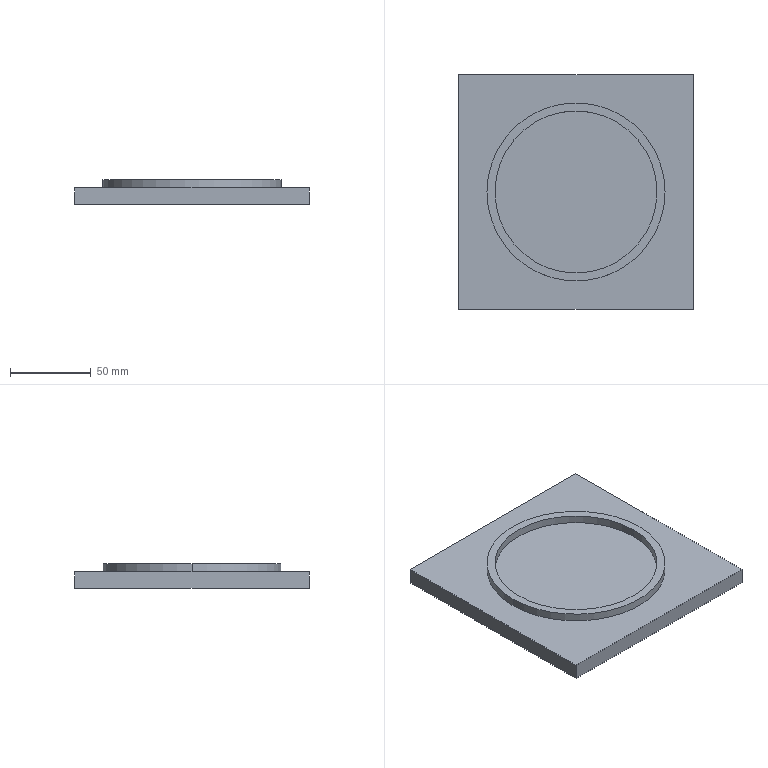Part | SolidWorks | features Extrusion 1, ICE 1 | 1 solid | 12 faces | box 145 x 145 x 15 mm | volume 218497 mm3 | plane 8 | cylinder 4 | commonest cylinder face diameters 100 x2 110 x2
STEP:
#1=CARTESIAN_POINT('',(22.5,72.5,15.));
#2=VERTEX_POINT('',#1);
#3=CARTESIAN_POINT('',(122.5,72.5,15.));
#4=VERTEX_POINT('',#3);
#5=CARTESIAN_POINT('',(72.5,72.5,15.));
#6=DIRECTION('',(0.,0.,1.));
#7=DIRECTION('',(1.,0.,0.));
#8=AXIS2_PLACEMENT_3D('',#5,#6,#7);
#9=CIRCLE('',#8,50.);
#10=EDGE_CURVE('',#2,#4,#9,.T.);
#11=ORIENTED_EDGE('',*,*,#10,.T.);
#12=CARTESIAN_POINT('',(122.5,72.5,10.));
#13=VERTEX_POINT('',#12);
#14=CARTESIAN_POINT('',(122.5,72.5,15.));
#15=DIRECTION('',(0.,0.,-1.));
#16=VECTOR('',#15,1000.);
#17=LINE('',#14,#16);
#18=EDGE_CURVE('',#4,#13,#17,.T.);
#19=ORIENTED_EDGE('',*,*,#18,.T.);
#20=CARTESIAN_POINT('',(22.5,72.5,10.));
#21=VERTEX_POINT('',#20);
#22=CARTESIAN_POINT('',(72.5,72.5,10.));
#23=DIRECTION('',(0.,0.,1.));
#24=DIRECTION('',(1.,0.,0.));
#25=AXIS2_PLACEMENT_3D('',#22,#23,#24);
#26=CIRCLE('',#25,50.);
#27=EDGE_CURVE('',#21,#13,#26,.T.);
#28=ORIENTED_EDGE('',*,*,#27,.F.);
#29=CARTESIAN_POINT('',(22.5,72.5,15.));
#30=DIRECTION('',(0.,0.,-1.));
#31=VECTOR('',#30,1000.);
#32=LINE('',#29,#31);
#33=EDGE_CURVE('',#2,#21,#32,.T.);
#34=ORIENTED_EDGE('',*,*,#33,.F.);
#35=EDGE_LOOP('',(#11,#19,#28,#34));
#36=FACE_OUTER_BOUND('',#35,.T.);
#37=CARTESIAN_POINT('',(72.5,72.5,15.));
#38=DIRECTION('',(0.,0.,-1.));
#39=DIRECTION('',(-1.,0.,0.));
#40=AXIS2_PLACEMENT_3D('',#37,#38,#39);
#41=CYLINDRICAL_SURFACE('',#40,50.);
#42=ADVANCED_FACE('',(#36),#41,.F.);
#43=CARTESIAN_POINT('',(127.5,72.5,15.));
#44=VERTEX_POINT('',#43);
#45=CARTESIAN_POINT('',(17.5,72.5,15.));
#46=VERTEX_POINT('',#45);
#47=CARTESIAN_POINT('',(72.5,72.5,15.));
#48=DIRECTION('',(0.,0.,1.));
#49=DIRECTION('',(1.,0.,0.));
#50=AXIS2_PLACEMENT_3D('',#47,#48,#49);
#51=CIRCLE('',#50,55.);
#52=EDGE_CURVE('',#44,#46,#51,.T.);
#53=ORIENTED_EDGE('',*,*,#52,.F.);
#54=CARTESIAN_POINT('',(127.5,72.5,10.));
#55=VERTEX_POINT('',#54);
#56=CARTESIAN_POINT('',(127.5,72.5,15.));
#57=DIRECTION('',(0.,0.,-1.));
#58=VECTOR('',#57,1000.);
#59=LINE('',#56,#58);
#60=EDGE_CURVE('',#44,#55,#59,.T.);
#61=ORIENTED_EDGE('',*,*,#60,.T.);
#62=CARTESIAN_POINT('',(17.5,72.5,10.));
#63=VERTEX_POINT('',#62);
#64=CARTESIAN_POINT('',(72.5,72.5,10.));
#65=DIRECTION('',(0.,0.,1.));
#66=DIRECTION('',(-1.,0.,0.));
#67=AXIS2_PLACEMENT_3D('',#64,#65,#66);
#68=CIRCLE('',#67,55.);
#69=EDGE_CURVE('',#55,#63,#68,.T.);
#70=ORIENTED_EDGE('',*,*,#69,.T.);
#71=CARTESIAN_POINT('',(17.5,72.5,15.));
#72=DIRECTION('',(0.,0.,-1.));
#73=VECTOR('',#72,1000.);
#74=LINE('',#71,#73);
#75=EDGE_CURVE('',#46,#63,#74,.T.);
#76=ORIENTED_EDGE('',*,*,#75,.F.);
#77=EDGE_LOOP('',(#53,#61,#70,#76));
#78=FACE_OUTER_BOUND('',#77,.T.);
#79=CARTESIAN_POINT('',(72.5,72.5,15.));
#80=DIRECTION('',(0.,0.,-1.));
#81=DIRECTION('',(-1.,0.,0.));
#82=AXIS2_PLACEMENT_3D('',#79,#80,#81);
#83=CYLINDRICAL_SURFACE('',#82,55.);
#84=ADVANCED_FACE('',(#78),#83,.T.);
#85=CARTESIAN_POINT('',(0.,145.,10.));
#86=VERTEX_POINT('',#85);
#87=CARTESIAN_POINT('',(0.,0.,10.));
#88=VERTEX_POINT('',#87);
#89=CARTESIAN_POINT('',(0.,0.,10.));
#90=DIRECTION('',(0.,-1.,0.));
#91=VECTOR('',#90,1000.);
#92=LINE('',#89,#91);
#93=EDGE_CURVE('',#86,#88,#92,.T.);
#94=ORIENTED_EDGE('',*,*,#93,.T.);
#95=CARTESIAN_POINT('',(145.,0.,10.));
#96=VERTEX_POINT('',#95);
#97=CARTESIAN_POINT('',(0.,0.,10.));
#98=DIRECTION('',(1.,0.,0.));
#99=VECTOR('',#98,1000.);
#100=LINE('',#97,#99);
#101=EDGE_CURVE('',#88,#96,#100,.T.);
#102=ORIENTED_EDGE('',*,*,#101,.T.);
#103=CARTESIAN_POINT('',(145.,145.,10.));
#104=VERTEX_POINT('',#103);
#105=CARTESIAN_POINT('',(145.,145.,10.));
#106=DIRECTION('',(0.,1.,0.));
#107=VECTOR('',#106,1000.);
#108=LINE('',#105,#107);
#109=EDGE_CURVE('',#96,#104,#108,.T.);
#110=ORIENTED_EDGE('',*,*,#109,.T.);
#111=CARTESIAN_POINT('',(0.,145.,10.));
#112=DIRECTION('',(-1.,0.,0.));
#113=VECTOR('',#112,1000.);
#114=LINE('',#111,#113);
#115=EDGE_CURVE('',#104,#86,#114,.T.);
#116=ORIENTED_EDGE('',*,*,#115,.T.);
#117=EDGE_LOOP('',(#94,#102,#110,#116));
#118=FACE_OUTER_BOUND('',#117,.T.);
#119=CARTESIAN_POINT('',(72.5,72.5,10.));
#120=DIRECTION('',(0.,0.,1.));
#121=DIRECTION('',(-1.,0.,0.));
#122=AXIS2_PLACEMENT_3D('',#119,#120,#121);
#123=CIRCLE('',#122,55.);
#124=EDGE_CURVE('',#63,#55,#123,.T.);
#125=ORIENTED_EDGE('',*,*,#124,.F.);
#126=ORIENTED_EDGE('',*,*,#69,.F.);
#127=EDGE_LOOP('',(#125,#126));
#128=FACE_BOUND('',#127,.T.);
#129=CARTESIAN_POINT('',(0.,145.,10.));
#130=DIRECTION('',(0.,0.,-1.));
#131=DIRECTION('',(-1.,0.,0.));
#132=AXIS2_PLACEMENT_3D('',#129,#130,#131);
#133=PLANE('',#132);
#134=ADVANCED_FACE('',(#118,#128),#133,.F.);
#135=CARTESIAN_POINT('',(0.,145.,0.));
#136=VERTEX_POINT('',#135);
#137=CARTESIAN_POINT('',(0.,0.,0.));
#138=VERTEX_POINT('',#137);
#139=CARTESIAN_POINT('',(0.,0.,0.));
#140=DIRECTION('',(0.,-1.,0.));
#141=VECTOR('',#140,1000.);
#142=LINE('',#139,#141);
#143=EDGE_CURVE('',#136,#138,#142,.T.);
#144=ORIENTED_EDGE('',*,*,#143,.T.);
#145=CARTESIAN_POINT('',(0.,0.,10.));
#146=DIRECTION('',(0.,0.,-1.));
#147=VECTOR('',#146,1000.);
#148=LINE('',#145,#147);
#149=EDGE_CURVE('',#88,#138,#148,.T.);
#150=ORIENTED_EDGE('',*,*,#149,.F.);
#151=ORIENTED_EDGE('',*,*,#93,.F.);
#152=CARTESIAN_POINT('',(0.,145.,10.));
#153=DIRECTION('',(0.,0.,-1.));
#154=VECTOR('',#153,1000.);
#155=LINE('',#152,#154);
#156=EDGE_CURVE('',#86,#136,#155,.T.);
#157=ORIENTED_EDGE('',*,*,#156,.T.);
#158=EDGE_LOOP('',(#144,#150,#151,#157));
#159=FACE_OUTER_BOUND('',#158,.T.);
#160=CARTESIAN_POINT('',(0.,0.,10.));
#161=DIRECTION('',(1.,0.,0.));
#162=DIRECTION('',(0.,0.,-1.));
#163=AXIS2_PLACEMENT_3D('',#160,#161,#162);
#164=PLANE('',#163);
#165=ADVANCED_FACE('',(#159),#164,.F.);
#166=CARTESIAN_POINT('',(145.,0.,0.));
#167=VERTEX_POINT('',#166);
#168=CARTESIAN_POINT('',(0.,0.,0.));
#169=DIRECTION('',(1.,0.,0.));
#170=VECTOR('',#169,1000.);
#171=LINE('',#168,#170);
#172=EDGE_CURVE('',#138,#167,#171,.T.);
#173=ORIENTED_EDGE('',*,*,#172,.T.);
#174=CARTESIAN_POINT('',(145.,0.,10.));
#175=DIRECTION('',(0.,0.,-1.));
#176=VECTOR('',#175,1000.);
#177=LINE('',#174,#176);
#178=EDGE_CURVE('',#96,#167,#177,.T.);
#179=ORIENTED_EDGE('',*,*,#178,.F.);
#180=ORIENTED_EDGE('',*,*,#101,.F.);
#181=ORIENTED_EDGE('',*,*,#149,.T.);
#182=EDGE_LOOP('',(#173,#179,#180,#181));
#183=FACE_OUTER_BOUND('',#182,.T.);
#184=CARTESIAN_POINT('',(0.,0.,10.));
#185=DIRECTION('',(0.,1.,0.));
#186=DIRECTION('',(0.,0.,1.));
#187=AXIS2_PLACEMENT_3D('',#184,#185,#186);
#188=PLANE('',#187);
#189=ADVANCED_FACE('',(#183),#188,.F.);
#190=CARTESIAN_POINT('',(145.,145.,0.));
#191=VERTEX_POINT('',#190);
#192=CARTESIAN_POINT('',(145.,145.,0.));
#193=DIRECTION('',(0.,1.,0.));
#194=VECTOR('',#193,1000.);
#195=LINE('',#192,#194);
#196=EDGE_CURVE('',#167,#191,#195,.T.);
#197=ORIENTED_EDGE('',*,*,#196,.T.);
#198=CARTESIAN_POINT('',(145.,145.,10.));
#199=DIRECTION('',(0.,0.,-1.));
#200=VECTOR('',#199,1000.);
#201=LINE('',#198,#200);
#202=EDGE_CURVE('',#104,#191,#201,.T.);
#203=ORIENTED_EDGE('',*,*,#202,.F.);
#204=ORIENTED_EDGE('',*,*,#109,.F.);
#205=ORIENTED_EDGE('',*,*,#178,.T.);
#206=EDGE_LOOP('',(#197,#203,#204,#205));
#207=FACE_OUTER_BOUND('',#206,.T.);
#208=CARTESIAN_POINT('',(145.,145.,10.));
#209=DIRECTION('',(-1.,0.,0.));
#210=DIRECTION('',(0.,-1.,0.));
#211=AXIS2_PLACEMENT_3D('',#208,#209,#210);
#212=PLANE('',#211);
#213=ADVANCED_FACE('',(#207),#212,.F.);
#214=CARTESIAN_POINT('',(0.,145.,0.));
#215=DIRECTION('',(-1.,0.,0.));
#216=VECTOR('',#215,1000.);
#217=LINE('',#214,#216);
#218=EDGE_CURVE('',#191,#136,#217,.T.);
#219=ORIENTED_EDGE('',*,*,#218,.T.);
#220=ORIENTED_EDGE('',*,*,#156,.F.);
#221=ORIENTED_EDGE('',*,*,#115,.F.);
#222=ORIENTED_EDGE('',*,*,#202,.T.);
#223=EDGE_LOOP('',(#219,#220,#221,#222));
#224=FACE_OUTER_BOUND('',#223,.T.);
#225=CARTESIAN_POINT('',(0.,145.,10.));
#226=DIRECTION('',(0.,-1.,0.));
#227=DIRECTION('',(0.,0.,-1.));
#228=AXIS2_PLACEMENT_3D('',#225,#226,#227);
#229=PLANE('',#228);
#230=ADVANCED_FACE('',(#224),#229,.F.);
#231=ORIENTED_EDGE('',*,*,#143,.F.);
#232=ORIENTED_EDGE('',*,*,#218,.F.);
#233=ORIENTED_EDGE('',*,*,#196,.F.);
#234=ORIENTED_EDGE('',*,*,#172,.F.);
#235=EDGE_LOOP('',(#231,#232,#233,#234));
#236=FACE_OUTER_BOUND('',#235,.T.);
#237=CARTESIAN_POINT('',(0.,145.,0.));
#238=DIRECTION('',(0.,0.,-1.));
#239=DIRECTION('',(-1.,0.,0.));
#240=AXIS2_PLACEMENT_3D('',#237,#238,#239);
#241=PLANE('',#240);
#242=ADVANCED_FACE('',(#236),#241,.T.);
#243=CARTESIAN_POINT('',(72.5,72.5,15.));
#244=DIRECTION('',(0.,0.,1.));
#245=DIRECTION('',(1.,0.,0.));
#246=AXIS2_PLACEMENT_3D('',#243,#244,#245);
#247=CIRCLE('',#246,55.);
#248=EDGE_CURVE('',#46,#44,#247,.T.);
#249=ORIENTED_EDGE('',*,*,#248,.T.);
#250=ORIENTED_EDGE('',*,*,#52,.T.);
#251=EDGE_LOOP('',(#249,#250));
#252=FACE_OUTER_BOUND('',#251,.T.);
#253=ORIENTED_EDGE('',*,*,#10,.F.);
#254=CARTESIAN_POINT('',(72.5,72.5,15.));
#255=DIRECTION('',(0.,0.,1.));
#256=DIRECTION('',(1.,0.,0.));
#257=AXIS2_PLACEMENT_3D('',#254,#255,#256);
#258=CIRCLE('',#257,50.);
#259=EDGE_CURVE('',#4,#2,#258,.T.);
#260=ORIENTED_EDGE('',*,*,#259,.F.);
#261=EDGE_LOOP('',(#253,#260));
#262=FACE_BOUND('',#261,.T.);
#263=CARTESIAN_POINT('',(72.5,72.5,15.));
#264=DIRECTION('',(0.,0.,1.));
#265=DIRECTION('',(1.,0.,0.));
#266=AXIS2_PLACEMENT_3D('',#263,#264,#265);
#267=PLANE('',#266);
#268=ADVANCED_FACE('',(#252,#262),#267,.T.);
#269=ORIENTED_EDGE('',*,*,#60,.F.);
#270=ORIENTED_EDGE('',*,*,#248,.F.);
#271=ORIENTED_EDGE('',*,*,#75,.T.);
#272=ORIENTED_EDGE('',*,*,#124,.T.);
#273=EDGE_LOOP('',(#269,#270,#271,#272));
#274=FACE_OUTER_BOUND('',#273,.T.);
#275=CARTESIAN_POINT('',(72.5,72.5,15.));
#276=DIRECTION('',(0.,0.,-1.));
#277=DIRECTION('',(-1.,0.,0.));
#278=AXIS2_PLACEMENT_3D('',#275,#276,#277);
#279=CYLINDRICAL_SURFACE('',#278,55.);
#280=ADVANCED_FACE('',(#274),#279,.T.);
#281=ORIENTED_EDGE('',*,*,#18,.F.);
#282=ORIENTED_EDGE('',*,*,#259,.T.);
#283=ORIENTED_EDGE('',*,*,#33,.T.);
#284=CARTESIAN_POINT('',(72.5,72.5,10.));
#285=DIRECTION('',(0.,0.,1.));
#286=DIRECTION('',(1.,0.,0.));
#287=AXIS2_PLACEMENT_3D('',#284,#285,#286);
#288=CIRCLE('',#287,50.);
#289=EDGE_CURVE('',#13,#21,#288,.T.);
#290=ORIENTED_EDGE('',*,*,#289,.F.);
#291=EDGE_LOOP('',(#281,#282,#283,#290));
#292=FACE_OUTER_BOUND('',#291,.T.);
#293=CARTESIAN_POINT('',(72.5,72.5,15.));
#294=DIRECTION('',(0.,0.,-1.));
#295=DIRECTION('',(-1.,0.,0.));
#296=AXIS2_PLACEMENT_3D('',#293,#294,#295);
#297=CYLINDRICAL_SURFACE('',#296,50.);
#298=ADVANCED_FACE('',(#292),#297,.F.);
#299=ORIENTED_EDGE('',*,*,#27,.T.);
#300=ORIENTED_EDGE('',*,*,#289,.T.);
#301=EDGE_LOOP('',(#299,#300));
#302=FACE_OUTER_BOUND('',#301,.T.);
#303=CARTESIAN_POINT('',(0.,145.,10.));
#304=DIRECTION('',(0.,0.,-1.));
#305=DIRECTION('',(-1.,0.,0.));
#306=AXIS2_PLACEMENT_3D('',#303,#304,#305);
#307=PLANE('',#306);
#308=ADVANCED_FACE('',(#302),#307,.F.);
#309=CLOSED_SHELL('',(#42,#84,#134,#165,#189,#213,#230,#242,#268,#280,#298,#308));
#310=MANIFOLD_SOLID_BREP('',#309);
#311=CARTESIAN_POINT('',(0.,0.,0.));
#312=DIRECTION('',(0.,0.,1.));
#313=DIRECTION('',(1.,0.,0.));
#314=AXIS2_PLACEMENT_3D('',#311,#312,#313);
#315=(LENGTH_UNIT()NAMED_UNIT(*)SI_UNIT(.MILLI.,.METRE.));
#316=UNCERTAINTY_MEASURE_WITH_UNIT(LENGTH_MEASURE(0.00001),#315,'','');
#317=(NAMED_UNIT(*)PLANE_ANGLE_UNIT()SI_UNIT($,.RADIAN.));
#318=(NAMED_UNIT(*)SI_UNIT($,.STERADIAN.)SOLID_ANGLE_UNIT());
#319=(GEOMETRIC_REPRESENTATION_CONTEXT(3)GLOBAL_UNCERTAINTY_ASSIGNED_CONTEXT((#316))GLOBAL_UNIT_ASSIGNED_CONTEXT((#315,#317,#318))REPRESENTATION_CONTEXT('',''));
#320=ADVANCED_BREP_SHAPE_REPRESENTATION('',(#310,#314),#319);